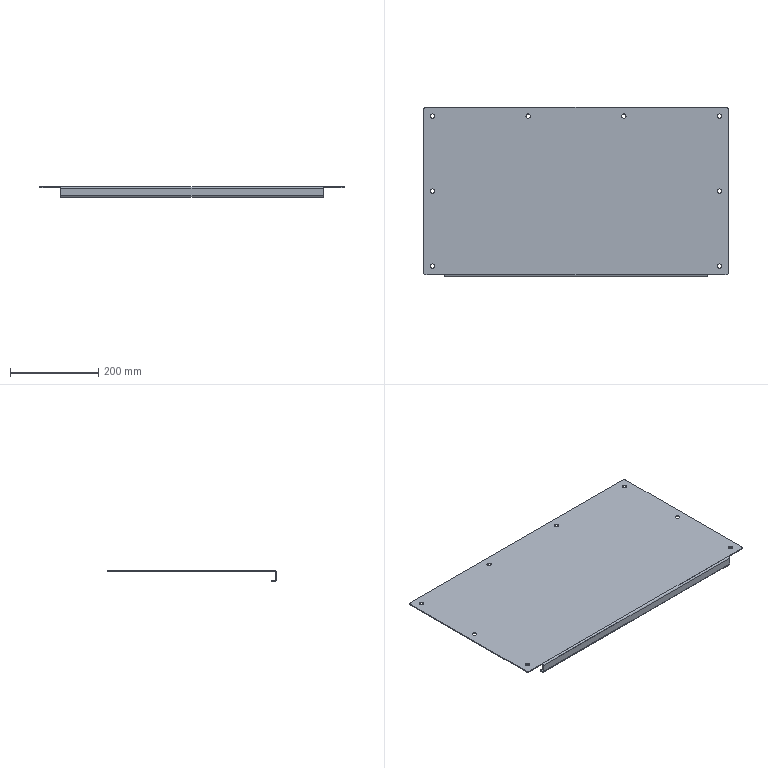Part | STEP file | 750038472 | 1 solid | 40 faces | box 690 x 384 x 24 mm | volume 562921 mm3 | cylinder 26 | plane 14 | commonest cylinder face diameters 10 x22 4 x2 8 x2
STEP:
#1=CARTESIAN_POINT('',(320.,360.,0.));
#2=VERTEX_POINT('',#1);
#3=CARTESIAN_POINT('',(330.,360.,0.));
#4=VERTEX_POINT('',#3);
#5=CARTESIAN_POINT('',(325.,360.,0.));
#6=DIRECTION('',(0.,0.,1.));
#7=DIRECTION('',(1.,0.,0.));
#8=AXIS2_PLACEMENT_3D('',#5,#6,#7);
#9=CIRCLE('',#8,5.);
#10=EDGE_CURVE('',#2,#4,#9,.T.);
#11=ORIENTED_EDGE('',*,*,#10,.F.);
#12=CARTESIAN_POINT('',(320.,360.,2.));
#13=VERTEX_POINT('',#12);
#14=CARTESIAN_POINT('',(320.,360.,-788.02));
#15=DIRECTION('',(0.,0.,1.));
#16=VECTOR('',#15,1000.);
#17=LINE('',#14,#16);
#18=EDGE_CURVE('',#2,#13,#17,.T.);
#19=ORIENTED_EDGE('',*,*,#18,.T.);
#20=CARTESIAN_POINT('',(330.,360.,2.));
#21=VERTEX_POINT('',#20);
#22=CARTESIAN_POINT('',(325.,360.,2.));
#23=DIRECTION('',(0.,0.,-1.));
#24=DIRECTION('',(1.,0.,0.));
#25=AXIS2_PLACEMENT_3D('',#22,#23,#24);
#26=CIRCLE('',#25,5.);
#27=EDGE_CURVE('',#21,#13,#26,.T.);
#28=ORIENTED_EDGE('',*,*,#27,.F.);
#29=CARTESIAN_POINT('',(330.,360.,-788.02));
#30=DIRECTION('',(0.,0.,1.));
#31=VECTOR('',#30,1000.);
#32=LINE('',#29,#31);
#33=EDGE_CURVE('',#4,#21,#32,.T.);
#34=ORIENTED_EDGE('',*,*,#33,.F.);
#35=EDGE_LOOP('',(#11,#19,#28,#34));
#36=FACE_OUTER_BOUND('',#35,.T.);
#37=CARTESIAN_POINT('',(325.,360.,-788.02));
#38=DIRECTION('',(0.,0.,1.));
#39=DIRECTION('',(1.,0.,0.));
#40=AXIS2_PLACEMENT_3D('',#37,#38,#39);
#41=CYLINDRICAL_SURFACE('',#40,5.);
#42=ADVANCED_FACE('',(#36),#41,.F.);
#43=CARTESIAN_POINT('',(320.,190.,0.));
#44=VERTEX_POINT('',#43);
#45=CARTESIAN_POINT('',(330.,190.,0.));
#46=VERTEX_POINT('',#45);
#47=CARTESIAN_POINT('',(325.,190.,0.));
#48=DIRECTION('',(0.,0.,1.));
#49=DIRECTION('',(1.,0.,0.));
#50=AXIS2_PLACEMENT_3D('',#47,#48,#49);
#51=CIRCLE('',#50,5.);
#52=EDGE_CURVE('',#44,#46,#51,.T.);
#53=ORIENTED_EDGE('',*,*,#52,.F.);
#54=CARTESIAN_POINT('',(320.,190.,2.));
#55=VERTEX_POINT('',#54);
#56=CARTESIAN_POINT('',(320.,190.,-788.02));
#57=DIRECTION('',(0.,0.,1.));
#58=VECTOR('',#57,1000.);
#59=LINE('',#56,#58);
#60=EDGE_CURVE('',#44,#55,#59,.T.);
#61=ORIENTED_EDGE('',*,*,#60,.T.);
#62=CARTESIAN_POINT('',(330.,190.,2.));
#63=VERTEX_POINT('',#62);
#64=CARTESIAN_POINT('',(325.,190.,2.));
#65=DIRECTION('',(0.,0.,-1.));
#66=DIRECTION('',(1.,0.,0.));
#67=AXIS2_PLACEMENT_3D('',#64,#65,#66);
#68=CIRCLE('',#67,5.);
#69=EDGE_CURVE('',#63,#55,#68,.T.);
#70=ORIENTED_EDGE('',*,*,#69,.F.);
#71=CARTESIAN_POINT('',(330.,190.,-788.02));
#72=DIRECTION('',(0.,0.,1.));
#73=VECTOR('',#72,1000.);
#74=LINE('',#71,#73);
#75=EDGE_CURVE('',#46,#63,#74,.T.);
#76=ORIENTED_EDGE('',*,*,#75,.F.);
#77=EDGE_LOOP('',(#53,#61,#70,#76));
#78=FACE_OUTER_BOUND('',#77,.T.);
#79=CARTESIAN_POINT('',(325.,190.,-788.02));
#80=DIRECTION('',(0.,0.,1.));
#81=DIRECTION('',(1.,0.,0.));
#82=AXIS2_PLACEMENT_3D('',#79,#80,#81);
#83=CYLINDRICAL_SURFACE('',#82,5.);
#84=ADVANCED_FACE('',(#78),#83,.F.);
#85=CARTESIAN_POINT('',(320.,20.,0.));
#86=VERTEX_POINT('',#85);
#87=CARTESIAN_POINT('',(330.,20.,0.));
#88=VERTEX_POINT('',#87);
#89=CARTESIAN_POINT('',(325.,20.,0.));
#90=DIRECTION('',(0.,0.,1.));
#91=DIRECTION('',(1.,0.,0.));
#92=AXIS2_PLACEMENT_3D('',#89,#90,#91);
#93=CIRCLE('',#92,5.);
#94=EDGE_CURVE('',#86,#88,#93,.T.);
#95=ORIENTED_EDGE('',*,*,#94,.F.);
#96=CARTESIAN_POINT('',(320.,20.,2.));
#97=VERTEX_POINT('',#96);
#98=CARTESIAN_POINT('',(320.,20.,-788.02));
#99=DIRECTION('',(0.,0.,1.));
#100=VECTOR('',#99,1000.);
#101=LINE('',#98,#100);
#102=EDGE_CURVE('',#86,#97,#101,.T.);
#103=ORIENTED_EDGE('',*,*,#102,.T.);
#104=CARTESIAN_POINT('',(330.,20.,2.));
#105=VERTEX_POINT('',#104);
#106=CARTESIAN_POINT('',(325.,20.,2.));
#107=DIRECTION('',(0.,0.,-1.));
#108=DIRECTION('',(1.,0.,0.));
#109=AXIS2_PLACEMENT_3D('',#106,#107,#108);
#110=CIRCLE('',#109,5.);
#111=EDGE_CURVE('',#105,#97,#110,.T.);
#112=ORIENTED_EDGE('',*,*,#111,.F.);
#113=CARTESIAN_POINT('',(330.,20.,-788.02));
#114=DIRECTION('',(0.,0.,1.));
#115=VECTOR('',#114,1000.);
#116=LINE('',#113,#115);
#117=EDGE_CURVE('',#88,#105,#116,.T.);
#118=ORIENTED_EDGE('',*,*,#117,.F.);
#119=EDGE_LOOP('',(#95,#103,#112,#118));
#120=FACE_OUTER_BOUND('',#119,.T.);
#121=CARTESIAN_POINT('',(325.,20.,-788.02));
#122=DIRECTION('',(0.,0.,1.));
#123=DIRECTION('',(1.,0.,0.));
#124=AXIS2_PLACEMENT_3D('',#121,#122,#123);
#125=CYLINDRICAL_SURFACE('',#124,5.);
#126=ADVANCED_FACE('',(#120),#125,.F.);
#127=CARTESIAN_POINT('',(103.333,360.,0.));
#128=VERTEX_POINT('',#127);
#129=CARTESIAN_POINT('',(113.333,360.,0.));
#130=VERTEX_POINT('',#129);
#131=CARTESIAN_POINT('',(108.333,360.,0.));
#132=DIRECTION('',(0.,0.,1.));
#133=DIRECTION('',(1.,0.,0.));
#134=AXIS2_PLACEMENT_3D('',#131,#132,#133);
#135=CIRCLE('',#134,5.);
#136=EDGE_CURVE('',#128,#130,#135,.T.);
#137=ORIENTED_EDGE('',*,*,#136,.F.);
#138=CARTESIAN_POINT('',(103.333,360.,2.));
#139=VERTEX_POINT('',#138);
#140=CARTESIAN_POINT('',(103.333,360.,-788.02));
#141=DIRECTION('',(0.,0.,1.));
#142=VECTOR('',#141,1000.);
#143=LINE('',#140,#142);
#144=EDGE_CURVE('',#128,#139,#143,.T.);
#145=ORIENTED_EDGE('',*,*,#144,.T.);
#146=CARTESIAN_POINT('',(113.333,360.,2.));
#147=VERTEX_POINT('',#146);
#148=CARTESIAN_POINT('',(108.333,360.,2.));
#149=DIRECTION('',(0.,0.,-1.));
#150=DIRECTION('',(1.,0.,0.));
#151=AXIS2_PLACEMENT_3D('',#148,#149,#150);
#152=CIRCLE('',#151,5.);
#153=EDGE_CURVE('',#147,#139,#152,.T.);
#154=ORIENTED_EDGE('',*,*,#153,.F.);
#155=CARTESIAN_POINT('',(113.333,360.,-788.02));
#156=DIRECTION('',(0.,0.,1.));
#157=VECTOR('',#156,1000.);
#158=LINE('',#155,#157);
#159=EDGE_CURVE('',#130,#147,#158,.T.);
#160=ORIENTED_EDGE('',*,*,#159,.F.);
#161=EDGE_LOOP('',(#137,#145,#154,#160));
#162=FACE_OUTER_BOUND('',#161,.T.);
#163=CARTESIAN_POINT('',(108.333,360.,-788.02));
#164=DIRECTION('',(0.,0.,1.));
#165=DIRECTION('',(1.,0.,0.));
#166=AXIS2_PLACEMENT_3D('',#163,#164,#165);
#167=CYLINDRICAL_SURFACE('',#166,5.);
#168=ADVANCED_FACE('',(#162),#167,.F.);
#169=CARTESIAN_POINT('',(-113.333,360.,0.));
#170=VERTEX_POINT('',#169);
#171=CARTESIAN_POINT('',(-103.333,360.,0.));
#172=VERTEX_POINT('',#171);
#173=CARTESIAN_POINT('',(-108.333,360.,0.));
#174=DIRECTION('',(0.,0.,1.));
#175=DIRECTION('',(1.,0.,0.));
#176=AXIS2_PLACEMENT_3D('',#173,#174,#175);
#177=CIRCLE('',#176,5.);
#178=EDGE_CURVE('',#170,#172,#177,.T.);
#179=ORIENTED_EDGE('',*,*,#178,.F.);
#180=CARTESIAN_POINT('',(-113.333,360.,2.));
#181=VERTEX_POINT('',#180);
#182=CARTESIAN_POINT('',(-113.333,360.,-788.02));
#183=DIRECTION('',(0.,0.,1.));
#184=VECTOR('',#183,1000.);
#185=LINE('',#182,#184);
#186=EDGE_CURVE('',#170,#181,#185,.T.);
#187=ORIENTED_EDGE('',*,*,#186,.T.);
#188=CARTESIAN_POINT('',(-103.333,360.,2.));
#189=VERTEX_POINT('',#188);
#190=CARTESIAN_POINT('',(-108.333,360.,2.));
#191=DIRECTION('',(0.,0.,-1.));
#192=DIRECTION('',(1.,0.,0.));
#193=AXIS2_PLACEMENT_3D('',#190,#191,#192);
#194=CIRCLE('',#193,5.);
#195=EDGE_CURVE('',#189,#181,#194,.T.);
#196=ORIENTED_EDGE('',*,*,#195,.F.);
#197=CARTESIAN_POINT('',(-103.333,360.,-788.02));
#198=DIRECTION('',(0.,0.,1.));
#199=VECTOR('',#198,1000.);
#200=LINE('',#197,#199);
#201=EDGE_CURVE('',#172,#189,#200,.T.);
#202=ORIENTED_EDGE('',*,*,#201,.F.);
#203=EDGE_LOOP('',(#179,#187,#196,#202));
#204=FACE_OUTER_BOUND('',#203,.T.);
#205=CARTESIAN_POINT('',(-108.333,360.,-788.02));
#206=DIRECTION('',(0.,0.,1.));
#207=DIRECTION('',(1.,0.,0.));
#208=AXIS2_PLACEMENT_3D('',#205,#206,#207);
#209=CYLINDRICAL_SURFACE('',#208,5.);
#210=ADVANCED_FACE('',(#204),#209,.F.);
#211=CARTESIAN_POINT('',(-330.,360.,0.));
#212=VERTEX_POINT('',#211);
#213=CARTESIAN_POINT('',(-320.,360.,0.));
#214=VERTEX_POINT('',#213);
#215=CARTESIAN_POINT('',(-325.,360.,0.));
#216=DIRECTION('',(0.,0.,1.));
#217=DIRECTION('',(1.,0.,0.));
#218=AXIS2_PLACEMENT_3D('',#215,#216,#217);
#219=CIRCLE('',#218,5.);
#220=EDGE_CURVE('',#212,#214,#219,.T.);
#221=ORIENTED_EDGE('',*,*,#220,.F.);
#222=CARTESIAN_POINT('',(-330.,360.,2.));
#223=VERTEX_POINT('',#222);
#224=CARTESIAN_POINT('',(-330.,360.,-788.02));
#225=DIRECTION('',(0.,0.,1.));
#226=VECTOR('',#225,1000.);
#227=LINE('',#224,#226);
#228=EDGE_CURVE('',#212,#223,#227,.T.);
#229=ORIENTED_EDGE('',*,*,#228,.T.);
#230=CARTESIAN_POINT('',(-320.,360.,2.));
#231=VERTEX_POINT('',#230);
#232=CARTESIAN_POINT('',(-325.,360.,2.));
#233=DIRECTION('',(0.,0.,-1.));
#234=DIRECTION('',(1.,0.,0.));
#235=AXIS2_PLACEMENT_3D('',#232,#233,#234);
#236=CIRCLE('',#235,5.);
#237=EDGE_CURVE('',#231,#223,#236,.T.);
#238=ORIENTED_EDGE('',*,*,#237,.F.);
#239=CARTESIAN_POINT('',(-320.,360.,-788.02));
#240=DIRECTION('',(0.,0.,1.));
#241=VECTOR('',#240,1000.);
#242=LINE('',#239,#241);
#243=EDGE_CURVE('',#214,#231,#242,.T.);
#244=ORIENTED_EDGE('',*,*,#243,.F.);
#245=EDGE_LOOP('',(#221,#229,#238,#244));
#246=FACE_OUTER_BOUND('',#245,.T.);
#247=CARTESIAN_POINT('',(-325.,360.,-788.02));
#248=DIRECTION('',(0.,0.,1.));
#249=DIRECTION('',(1.,0.,0.));
#250=AXIS2_PLACEMENT_3D('',#247,#248,#249);
#251=CYLINDRICAL_SURFACE('',#250,5.);
#252=ADVANCED_FACE('',(#246),#251,.F.);
#253=CARTESIAN_POINT('',(-330.,190.,0.));
#254=VERTEX_POINT('',#253);
#255=CARTESIAN_POINT('',(-320.,190.,0.));
#256=VERTEX_POINT('',#255);
#257=CARTESIAN_POINT('',(-325.,190.,0.));
#258=DIRECTION('',(0.,0.,1.));
#259=DIRECTION('',(1.,0.,0.));
#260=AXIS2_PLACEMENT_3D('',#257,#258,#259);
#261=CIRCLE('',#260,5.);
#262=EDGE_CURVE('',#254,#256,#261,.T.);
#263=ORIENTED_EDGE('',*,*,#262,.F.);
#264=CARTESIAN_POINT('',(-330.,190.,2.));
#265=VERTEX_POINT('',#264);
#266=CARTESIAN_POINT('',(-330.,190.,-788.02));
#267=DIRECTION('',(0.,0.,1.));
#268=VECTOR('',#267,1000.);
#269=LINE('',#266,#268);
#270=EDGE_CURVE('',#254,#265,#269,.T.);
#271=ORIENTED_EDGE('',*,*,#270,.T.);
#272=CARTESIAN_POINT('',(-320.,190.,2.));
#273=VERTEX_POINT('',#272);
#274=CARTESIAN_POINT('',(-325.,190.,2.));
#275=DIRECTION('',(0.,0.,-1.));
#276=DIRECTION('',(1.,0.,0.));
#277=AXIS2_PLACEMENT_3D('',#274,#275,#276);
#278=CIRCLE('',#277,5.);
#279=EDGE_CURVE('',#273,#265,#278,.T.);
#280=ORIENTED_EDGE('',*,*,#279,.F.);
#281=CARTESIAN_POINT('',(-320.,190.,-788.02));
#282=DIRECTION('',(0.,0.,1.));
#283=VECTOR('',#282,1000.);
#284=LINE('',#281,#283);
#285=EDGE_CURVE('',#256,#273,#284,.T.);
#286=ORIENTED_EDGE('',*,*,#285,.F.);
#287=EDGE_LOOP('',(#263,#271,#280,#286));
#288=FACE_OUTER_BOUND('',#287,.T.);
#289=CARTESIAN_POINT('',(-325.,190.,-788.02));
#290=DIRECTION('',(0.,0.,1.));
#291=DIRECTION('',(1.,0.,0.));
#292=AXIS2_PLACEMENT_3D('',#289,#290,#291);
#293=CYLINDRICAL_SURFACE('',#292,5.);
#294=ADVANCED_FACE('',(#288),#293,.F.);
#295=CARTESIAN_POINT('',(-330.,20.,0.));
#296=VERTEX_POINT('',#295);
#297=CARTESIAN_POINT('',(-320.,20.,0.));
#298=VERTEX_POINT('',#297);
#299=CARTESIAN_POINT('',(-325.,20.,0.));
#300=DIRECTION('',(0.,0.,1.));
#301=DIRECTION('',(1.,0.,0.));
#302=AXIS2_PLACEMENT_3D('',#299,#300,#301);
#303=CIRCLE('',#302,5.);
#304=EDGE_CURVE('',#296,#298,#303,.T.);
#305=ORIENTED_EDGE('',*,*,#304,.F.);
#306=CARTESIAN_POINT('',(-330.,20.,2.));
#307=VERTEX_POINT('',#306);
#308=CARTESIAN_POINT('',(-330.,20.,-788.02));
#309=DIRECTION('',(0.,0.,1.));
#310=VECTOR('',#309,1000.);
#311=LINE('',#308,#310);
#312=EDGE_CURVE('',#296,#307,#311,.T.);
#313=ORIENTED_EDGE('',*,*,#312,.T.);
#314=CARTESIAN_POINT('',(-320.,20.,2.));
#315=VERTEX_POINT('',#314);
#316=CARTESIAN_POINT('',(-325.,20.,2.));
#317=DIRECTION('',(0.,0.,-1.));
#318=DIRECTION('',(1.,0.,0.));
#319=AXIS2_PLACEMENT_3D('',#316,#317,#318);
#320=CIRCLE('',#319,5.);
#321=EDGE_CURVE('',#315,#307,#320,.T.);
#322=ORIENTED_EDGE('',*,*,#321,.F.);
#323=CARTESIAN_POINT('',(-320.,20.,-788.02));
#324=DIRECTION('',(0.,0.,1.));
#325=VECTOR('',#324,1000.);
#326=LINE('',#323,#325);
#327=EDGE_CURVE('',#298,#315,#326,.T.);
#328=ORIENTED_EDGE('',*,*,#327,.F.);
#329=EDGE_LOOP('',(#305,#313,#322,#328));
#330=FACE_OUTER_BOUND('',#329,.T.);
#331=CARTESIAN_POINT('',(-325.,20.,-788.02));
#332=DIRECTION('',(0.,0.,1.));
#333=DIRECTION('',(1.,0.,0.));
#334=AXIS2_PLACEMENT_3D('',#331,#332,#333);
#335=CYLINDRICAL_SURFACE('',#334,5.);
#336=ADVANCED_FACE('',(#330),#335,.F.);
#337=CARTESIAN_POINT('',(345.,5.,2.));
#338=VERTEX_POINT('',#337);
#339=CARTESIAN_POINT('',(345.,375.,2.));
#340=VERTEX_POINT('',#339);
#341=CARTESIAN_POINT('',(345.,0.,2.));
#342=DIRECTION('',(0.,1.,0.));
#343=VECTOR('',#342,1000.);
#344=LINE('',#341,#343);
#345=EDGE_CURVE('',#338,#340,#344,.T.);
#346=ORIENTED_EDGE('',*,*,#345,.T.);
#347=CARTESIAN_POINT('',(340.,380.,2.));
#348=VERTEX_POINT('',#347);
#349=CARTESIAN_POINT('',(340.,375.,2.));
#350=DIRECTION('',(0.,0.,1.));
#351=DIRECTION('',(-1.,0.,0.));
#352=AXIS2_PLACEMENT_3D('',#349,#350,#351);
#353=CIRCLE('',#352,5.);
#354=EDGE_CURVE('',#340,#348,#353,.T.);
#355=ORIENTED_EDGE('',*,*,#354,.T.);
#356=CARTESIAN_POINT('',(-340.,380.,2.));
#357=VERTEX_POINT('',#356);
#358=CARTESIAN_POINT('',(0.,380.,2.));
#359=DIRECTION('',(-1.,0.,0.));
#360=VECTOR('',#359,1000.);
#361=LINE('',#358,#360);
#362=EDGE_CURVE('',#348,#357,#361,.T.);
#363=ORIENTED_EDGE('',*,*,#362,.T.);
#364=CARTESIAN_POINT('',(-345.,375.,2.));
#365=VERTEX_POINT('',#364);
#366=CARTESIAN_POINT('',(-340.,375.,2.));
#367=DIRECTION('',(0.,0.,1.));
#368=DIRECTION('',(-1.,0.,0.));
#369=AXIS2_PLACEMENT_3D('',#366,#367,#368);
#370=CIRCLE('',#369,5.);
#371=EDGE_CURVE('',#357,#365,#370,.T.);
#372=ORIENTED_EDGE('',*,*,#371,.T.);
#373=CARTESIAN_POINT('',(-345.,5.,2.));
#374=VERTEX_POINT('',#373);
#375=CARTESIAN_POINT('',(-345.,0.,2.));
#376=DIRECTION('',(0.,-1.,0.));
#377=VECTOR('',#376,1000.);
#378=LINE('',#375,#377);
#379=EDGE_CURVE('',#365,#374,#378,.T.);
#380=ORIENTED_EDGE('',*,*,#379,.T.);
#381=CARTESIAN_POINT('',(-340.,0.,2.));
#382=VERTEX_POINT('',#381);
#383=CARTESIAN_POINT('',(-340.,5.,2.));
#384=DIRECTION('',(0.,0.,1.));
#385=DIRECTION('',(-1.,0.,0.));
#386=AXIS2_PLACEMENT_3D('',#383,#384,#385);
#387=CIRCLE('',#386,5.);
#388=EDGE_CURVE('',#374,#382,#387,.T.);
#389=ORIENTED_EDGE('',*,*,#388,.T.);
#390=CARTESIAN_POINT('',(-298.,0.,2.));
#391=VERTEX_POINT('',#390);
#392=CARTESIAN_POINT('',(0.,0.,2.));
#393=DIRECTION('',(1.,0.,0.));
#394=VECTOR('',#393,1000.);
#395=LINE('',#392,#394);
#396=EDGE_CURVE('',#382,#391,#395,.T.);
#397=ORIENTED_EDGE('',*,*,#396,.T.);
#398=CARTESIAN_POINT('',(298.,0.,2.));
#399=VERTEX_POINT('',#398);
#400=CARTESIAN_POINT('',(0.,0.,2.));
#401=DIRECTION('',(1.,0.,0.));
#402=VECTOR('',#401,1000.);
#403=LINE('',#400,#402);
#404=EDGE_CURVE('',#391,#399,#403,.T.);
#405=ORIENTED_EDGE('',*,*,#404,.T.);
#406=CARTESIAN_POINT('',(340.,0.,2.));
#407=VERTEX_POINT('',#406);
#408=CARTESIAN_POINT('',(0.,0.,2.));
#409=DIRECTION('',(1.,0.,0.));
#410=VECTOR('',#409,1000.);
#411=LINE('',#408,#410);
#412=EDGE_CURVE('',#399,#407,#411,.T.);
#413=ORIENTED_EDGE('',*,*,#412,.T.);
#414=CARTESIAN_POINT('',(340.,5.,2.));
#415=DIRECTION('',(0.,0.,1.));
#416=DIRECTION('',(-1.,0.,0.));
#417=AXIS2_PLACEMENT_3D('',#414,#415,#416);
#418=CIRCLE('',#417,5.);
#419=EDGE_CURVE('',#407,#338,#418,.T.);
#420=ORIENTED_EDGE('',*,*,#419,.T.);
#421=EDGE_LOOP('',(#346,#355,#363,#372,#380,#389,#397,#405,#413,#420));
#422=FACE_OUTER_BOUND('',#421,.T.);
#423=ORIENTED_EDGE('',*,*,#27,.T.);
#424=CARTESIAN_POINT('',(325.,360.,2.));
#425=DIRECTION('',(0.,0.,-1.));
#426=DIRECTION('',(1.,0.,0.));
#427=AXIS2_PLACEMENT_3D('',#424,#425,#426);
#428=CIRCLE('',#427,5.);
#429=EDGE_CURVE('',#13,#21,#428,.T.);
#430=ORIENTED_EDGE('',*,*,#429,.T.);
#431=EDGE_LOOP('',(#423,#430));
#432=FACE_BOUND('',#431,.T.);
#433=ORIENTED_EDGE('',*,*,#69,.T.);
#434=CARTESIAN_POINT('',(325.,190.,2.));
#435=DIRECTION('',(0.,0.,-1.));
#436=DIRECTION('',(1.,0.,0.));
#437=AXIS2_PLACEMENT_3D('',#434,#435,#436);
#438=CIRCLE('',#437,5.);
#439=EDGE_CURVE('',#55,#63,#438,.T.);
#440=ORIENTED_EDGE('',*,*,#439,.T.);
#441=EDGE_LOOP('',(#433,#440));
#442=FACE_BOUND('',#441,.T.);
#443=ORIENTED_EDGE('',*,*,#111,.T.);
#444=CARTESIAN_POINT('',(325.,20.,2.));
#445=DIRECTION('',(0.,0.,-1.));
#446=DIRECTION('',(1.,0.,0.));
#447=AXIS2_PLACEMENT_3D('',#444,#445,#446);
#448=CIRCLE('',#447,5.);
#449=EDGE_CURVE('',#97,#105,#448,.T.);
#450=ORIENTED_EDGE('',*,*,#449,.T.);
#451=EDGE_LOOP('',(#443,#450));
#452=FACE_BOUND('',#451,.T.);
#453=ORIENTED_EDGE('',*,*,#153,.T.);
#454=CARTESIAN_POINT('',(108.333,360.,2.));
#455=DIRECTION('',(0.,0.,-1.));
#456=DIRECTION('',(1.,0.,0.));
#457=AXIS2_PLACEMENT_3D('',#454,#455,#456);
#458=CIRCLE('',#457,5.);
#459=EDGE_CURVE('',#139,#147,#458,.T.);
#460=ORIENTED_EDGE('',*,*,#459,.T.);
#461=EDGE_LOOP('',(#453,#460));
#462=FACE_BOUND('',#461,.T.);
#463=ORIENTED_EDGE('',*,*,#195,.T.);
#464=CARTESIAN_POINT('',(-108.333,360.,2.));
#465=DIRECTION('',(0.,0.,-1.));
#466=DIRECTION('',(1.,0.,0.));
#467=AXIS2_PLACEMENT_3D('',#464,#465,#466);
#468=CIRCLE('',#467,5.);
#469=EDGE_CURVE('',#181,#189,#468,.T.);
#470=ORIENTED_EDGE('',*,*,#469,.T.);
#471=EDGE_LOOP('',(#463,#470));
#472=FACE_BOUND('',#471,.T.);
#473=ORIENTED_EDGE('',*,*,#237,.T.);
#474=CARTESIAN_POINT('',(-325.,360.,2.));
#475=DIRECTION('',(0.,0.,-1.));
#476=DIRECTION('',(1.,0.,0.));
#477=AXIS2_PLACEMENT_3D('',#474,#475,#476);
#478=CIRCLE('',#477,5.);
#479=EDGE_CURVE('',#223,#231,#478,.T.);
#480=ORIENTED_EDGE('',*,*,#479,.T.);
#481=EDGE_LOOP('',(#473,#480));
#482=FACE_BOUND('',#481,.T.);
#483=ORIENTED_EDGE('',*,*,#279,.T.);
#484=CARTESIAN_POINT('',(-325.,190.,2.));
#485=DIRECTION('',(0.,0.,-1.));
#486=DIRECTION('',(1.,0.,0.));
#487=AXIS2_PLACEMENT_3D('',#484,#485,#486);
#488=CIRCLE('',#487,5.);
#489=EDGE_CURVE('',#265,#273,#488,.T.);
#490=ORIENTED_EDGE('',*,*,#489,.T.);
#491=EDGE_LOOP('',(#483,#490));
#492=FACE_BOUND('',#491,.T.);
#493=ORIENTED_EDGE('',*,*,#321,.T.);
#494=CARTESIAN_POINT('',(-325.,20.,2.));
#495=DIRECTION('',(0.,0.,-1.));
#496=DIRECTION('',(1.,0.,0.));
#497=AXIS2_PLACEMENT_3D('',#494,#495,#496);
#498=CIRCLE('',#497,5.);
#499=EDGE_CURVE('',#307,#315,#498,.T.);
#500=ORIENTED_EDGE('',*,*,#499,.T.);
#501=EDGE_LOOP('',(#493,#500));
#502=FACE_BOUND('',#501,.T.);
#503=CARTESIAN_POINT('',(0.,0.,2.));
#504=DIRECTION('',(0.,0.,1.));
#505=DIRECTION('',(1.,0.,0.));
#506=AXIS2_PLACEMENT_3D('',#503,#504,#505);
#507=PLANE('',#506);
#508=ADVANCED_FACE('',(#422,#432,#442,#452,#462,#472,#482,#492,#502),#507,.T.);
#509=CARTESIAN_POINT('',(345.,375.,0.));
#510=VERTEX_POINT('',#509);
#511=CARTESIAN_POINT('',(340.,380.,0.));
#512=VERTEX_POINT('',#511);
#513=CARTESIAN_POINT('',(340.,375.,0.));
#514=DIRECTION('',(0.,0.,1.));
#515=DIRECTION('',(-1.,0.,0.));
#516=AXIS2_PLACEMENT_3D('',#513,#514,#515);
#517=CIRCLE('',#516,5.);
#518=EDGE_CURVE('',#510,#512,#517,.T.);
#519=ORIENTED_EDGE('',*,*,#518,.T.);
#520=CARTESIAN_POINT('',(340.,380.,2.));
#521=DIRECTION('',(0.,0.,1.));
#522=VECTOR('',#521,1000.);
#523=LINE('',#520,#522);
#524=EDGE_CURVE('',#512,#348,#523,.T.);
#525=ORIENTED_EDGE('',*,*,#524,.T.);
#526=ORIENTED_EDGE('',*,*,#354,.F.);
#527=CARTESIAN_POINT('',(345.,375.,2.));
#528=DIRECTION('',(0.,0.,-1.));
#529=VECTOR('',#528,1000.);
#530=LINE('',#527,#529);
#531=EDGE_CURVE('',#340,#510,#530,.T.);
#532=ORIENTED_EDGE('',*,*,#531,.T.);
#533=EDGE_LOOP('',(#519,#525,#526,#532));
#534=FACE_OUTER_BOUND('',#533,.T.);
#535=CARTESIAN_POINT('',(340.,375.,2.));
#536=DIRECTION('',(0.,0.,-1.));
#537=DIRECTION('',(-1.,0.,0.));
#538=AXIS2_PLACEMENT_3D('',#535,#536,#537);
#539=CYLINDRICAL_SURFACE('',#538,5.);
#540=ADVANCED_FACE('',(#534),#539,.T.);
#541=CARTESIAN_POINT('',(345.,5.,0.));
#542=VERTEX_POINT('',#541);
#543=CARTESIAN_POINT('',(345.,5.,2.));
#544=DIRECTION('',(0.,0.,1.));
#545=VECTOR('',#544,1000.);
#546=LINE('',#543,#545);
#547=EDGE_CURVE('',#542,#338,#546,.T.);
#548=ORIENTED_EDGE('',*,*,#547,.F.);
#549=CARTESIAN_POINT('',(345.,0.,0.));
#550=DIRECTION('',(0.,-1.,0.));
#551=VECTOR('',#550,1000.);
#552=LINE('',#549,#551);
#553=EDGE_CURVE('',#510,#542,#552,.T.);
#554=ORIENTED_EDGE('',*,*,#553,.F.);
#555=ORIENTED_EDGE('',*,*,#531,.F.);
#556=ORIENTED_EDGE('',*,*,#345,.F.);
#557=EDGE_LOOP('',(#548,#554,#555,#556));
#558=FACE_OUTER_BOUND('',#557,.T.);
#559=CARTESIAN_POINT('',(345.,0.,2.));
#560=DIRECTION('',(-1.,0.,0.));
#561=DIRECTION('',(0.,-1.,0.));
#562=AXIS2_PLACEMENT_3D('',#559,#560,#561);
#563=PLANE('',#562);
#564=ADVANCED_FACE('',(#558),#563,.F.);
#565=CARTESIAN_POINT('',(340.,0.,0.));
#566=VERTEX_POINT('',#565);
#567=CARTESIAN_POINT('',(340.,5.,0.));
#568=DIRECTION('',(0.,0.,1.));
#569=DIRECTION('',(-1.,0.,0.));
#570=AXIS2_PLACEMENT_3D('',#567,#568,#569);
#571=CIRCLE('',#570,5.);
#572=EDGE_CURVE('',#566,#542,#571,.T.);
#573=ORIENTED_EDGE('',*,*,#572,.T.);
#574=ORIENTED_EDGE('',*,*,#547,.T.);
#575=ORIENTED_EDGE('',*,*,#419,.F.);
#576=CARTESIAN_POINT('',(340.,0.,2.));
#577=DIRECTION('',(0.,0.,-1.));
#578=VECTOR('',#577,1000.);
#579=LINE('',#576,#578);
#580=EDGE_CURVE('',#407,#566,#579,.T.);
#581=ORIENTED_EDGE('',*,*,#580,.T.);
#582=EDGE_LOOP('',(#573,#574,#575,#581));
#583=FACE_OUTER_BOUND('',#582,.T.);
#584=CARTESIAN_POINT('',(340.,5.,2.));
#585=DIRECTION('',(0.,0.,-1.));
#586=DIRECTION('',(-1.,0.,0.));
#587=AXIS2_PLACEMENT_3D('',#584,#585,#586);
#588=CYLINDRICAL_SURFACE('',#587,5.);
#589=ADVANCED_FACE('',(#583),#588,.T.);
#590=ORIENTED_EDGE('',*,*,#580,.F.);
#591=ORIENTED_EDGE('',*,*,#412,.F.);
#592=CARTESIAN_POINT('',(298.,0.,0.));
#593=VERTEX_POINT('',#592);
#594=CARTESIAN_POINT('',(298.,0.,2.));
#595=DIRECTION('',(0.,0.,1.));
#596=VECTOR('',#595,1000.);
#597=LINE('',#594,#596);
#598=EDGE_CURVE('',#593,#399,#597,.T.);
#599=ORIENTED_EDGE('',*,*,#598,.F.);
#600=CARTESIAN_POINT('',(-345.,0.,0.));
#601=DIRECTION('',(-1.,0.,0.));
#602=VECTOR('',#601,1000.);
#603=LINE('',#600,#602);
#604=EDGE_CURVE('',#566,#593,#603,.T.);
#605=ORIENTED_EDGE('',*,*,#604,.F.);
#606=EDGE_LOOP('',(#590,#591,#599,#605));
#607=FACE_OUTER_BOUND('',#606,.T.);
#608=CARTESIAN_POINT('',(-345.,0.,2.));
#609=DIRECTION('',(0.,1.,0.));
#610=DIRECTION('',(0.,0.,1.));
#611=AXIS2_PLACEMENT_3D('',#608,#609,#610);
#612=PLANE('',#611);
#613=ADVANCED_FACE('',(#607),#612,.F.);
#614=CARTESIAN_POINT('',(298.,-4.,-2.));
#615=VERTEX_POINT('',#614);
#616=CARTESIAN_POINT('',(298.,0.,-2.));
#617=DIRECTION('',(-1.,0.,0.));
#618=DIRECTION('',(0.,0.,1.));
#619=AXIS2_PLACEMENT_3D('',#616,#617,#618);
#620=CIRCLE('',#619,4.);
#621=EDGE_CURVE('',#615,#399,#620,.T.);
#622=ORIENTED_EDGE('',*,*,#621,.T.);
#623=ORIENTED_EDGE('',*,*,#404,.F.);
#624=CARTESIAN_POINT('',(-298.,-4.,-2.));
#625=VERTEX_POINT('',#624);
#626=CARTESIAN_POINT('',(-298.,0.,-2.));
#627=DIRECTION('',(1.,0.,0.));
#628=DIRECTION('',(0.,0.,1.));
#629=AXIS2_PLACEMENT_3D('',#626,#627,#628);
#630=CIRCLE('',#629,4.);
#631=EDGE_CURVE('',#391,#625,#630,.T.);
#632=ORIENTED_EDGE('',*,*,#631,.T.);
#633=CARTESIAN_POINT('',(298.,-4.,-2.));
#634=DIRECTION('',(1.,0.,0.));
#635=VECTOR('',#634,1000.);
#636=LINE('',#633,#635);
#637=EDGE_CURVE('',#625,#615,#636,.T.);
#638=ORIENTED_EDGE('',*,*,#637,.T.);
#639=EDGE_LOOP('',(#622,#623,#632,#638));
#640=FACE_OUTER_BOUND('',#639,.T.);
#641=CARTESIAN_POINT('',(298.,0.,-2.));
#642=DIRECTION('',(-1.,0.,0.));
#643=DIRECTION('',(0.,0.,1.));
#644=AXIS2_PLACEMENT_3D('',#641,#642,#643);
#645=CYLINDRICAL_SURFACE('',#644,4.);
#646=ADVANCED_FACE('',(#640),#645,.T.);
#647=CARTESIAN_POINT('',(-340.,0.,0.));
#648=VERTEX_POINT('',#647);
#649=CARTESIAN_POINT('',(-340.,0.,2.));
#650=DIRECTION('',(0.,0.,1.));
#651=VECTOR('',#650,1000.);
#652=LINE('',#649,#651);
#653=EDGE_CURVE('',#648,#382,#652,.T.);
#654=ORIENTED_EDGE('',*,*,#653,.F.);
#655=CARTESIAN_POINT('',(-298.,0.,0.));
#656=VERTEX_POINT('',#655);
#657=CARTESIAN_POINT('',(-345.,0.,0.));
#658=DIRECTION('',(-1.,0.,0.));
#659=VECTOR('',#658,1000.);
#660=LINE('',#657,#659);
#661=EDGE_CURVE('',#656,#648,#660,.T.);
#662=ORIENTED_EDGE('',*,*,#661,.F.);
#663=CARTESIAN_POINT('',(-298.,0.,2.));
#664=DIRECTION('',(0.,0.,-1.));
#665=VECTOR('',#664,1000.);
#666=LINE('',#663,#665);
#667=EDGE_CURVE('',#391,#656,#666,.T.);
#668=ORIENTED_EDGE('',*,*,#667,.F.);
#669=ORIENTED_EDGE('',*,*,#396,.F.);
#670=EDGE_LOOP('',(#654,#662,#668,#669));
#671=FACE_OUTER_BOUND('',#670,.T.);
#672=CARTESIAN_POINT('',(-345.,0.,2.));
#673=DIRECTION('',(0.,1.,0.));
#674=DIRECTION('',(0.,0.,1.));
#675=AXIS2_PLACEMENT_3D('',#672,#673,#674);
#676=PLANE('',#675);
#677=ADVANCED_FACE('',(#671),#676,.F.);
#678=CARTESIAN_POINT('',(-345.,5.,0.));
#679=VERTEX_POINT('',#678);
#680=CARTESIAN_POINT('',(-340.,5.,0.));
#681=DIRECTION('',(0.,0.,1.));
#682=DIRECTION('',(-1.,0.,0.));
#683=AXIS2_PLACEMENT_3D('',#680,#681,#682);
#684=CIRCLE('',#683,5.);
#685=EDGE_CURVE('',#679,#648,#684,.T.);
#686=ORIENTED_EDGE('',*,*,#685,.T.);
#687=ORIENTED_EDGE('',*,*,#653,.T.);
#688=ORIENTED_EDGE('',*,*,#388,.F.);
#689=CARTESIAN_POINT('',(-345.,5.,2.));
#690=DIRECTION('',(0.,0.,-1.));
#691=VECTOR('',#690,1000.);
#692=LINE('',#689,#691);
#693=EDGE_CURVE('',#374,#679,#692,.T.);
#694=ORIENTED_EDGE('',*,*,#693,.T.);
#695=EDGE_LOOP('',(#686,#687,#688,#694));
#696=FACE_OUTER_BOUND('',#695,.T.);
#697=CARTESIAN_POINT('',(-340.,5.,2.));
#698=DIRECTION('',(0.,0.,-1.));
#699=DIRECTION('',(-1.,0.,0.));
#700=AXIS2_PLACEMENT_3D('',#697,#698,#699);
#701=CYLINDRICAL_SURFACE('',#700,5.);
#702=ADVANCED_FACE('',(#696),#701,.T.);
#703=CARTESIAN_POINT('',(-345.,375.,0.));
#704=VERTEX_POINT('',#703);
#705=CARTESIAN_POINT('',(-345.,375.,2.));
#706=DIRECTION('',(0.,0.,1.));
#707=VECTOR('',#706,1000.);
#708=LINE('',#705,#707);
#709=EDGE_CURVE('',#704,#365,#708,.T.);
#710=ORIENTED_EDGE('',*,*,#709,.F.);
#711=CARTESIAN_POINT('',(-345.,380.,0.));
#712=DIRECTION('',(0.,1.,0.));
#713=VECTOR('',#712,1000.);
#714=LINE('',#711,#713);
#715=EDGE_CURVE('',#679,#704,#714,.T.);
#716=ORIENTED_EDGE('',*,*,#715,.F.);
#717=ORIENTED_EDGE('',*,*,#693,.F.);
#718=ORIENTED_EDGE('',*,*,#379,.F.);
#719=EDGE_LOOP('',(#710,#716,#717,#718));
#720=FACE_OUTER_BOUND('',#719,.T.);
#721=CARTESIAN_POINT('',(-345.,380.,2.));
#722=DIRECTION('',(1.,0.,0.));
#723=DIRECTION('',(0.,1.,0.));
#724=AXIS2_PLACEMENT_3D('',#721,#722,#723);
#725=PLANE('',#724);
#726=ADVANCED_FACE('',(#720),#725,.F.);
#727=CARTESIAN_POINT('',(-340.,380.,0.));
#728=VERTEX_POINT('',#727);
#729=CARTESIAN_POINT('',(-340.,375.,0.));
#730=DIRECTION('',(0.,0.,1.));
#731=DIRECTION('',(-1.,0.,0.));
#732=AXIS2_PLACEMENT_3D('',#729,#730,#731);
#733=CIRCLE('',#732,5.);
#734=EDGE_CURVE('',#728,#704,#733,.T.);
#735=ORIENTED_EDGE('',*,*,#734,.T.);
#736=ORIENTED_EDGE('',*,*,#709,.T.);
#737=ORIENTED_EDGE('',*,*,#371,.F.);
#738=CARTESIAN_POINT('',(-340.,380.,2.));
#739=DIRECTION('',(0.,0.,-1.));
#740=VECTOR('',#739,1000.);
#741=LINE('',#738,#740);
#742=EDGE_CURVE('',#357,#728,#741,.T.);
#743=ORIENTED_EDGE('',*,*,#742,.T.);
#744=EDGE_LOOP('',(#735,#736,#737,#743));
#745=FACE_OUTER_BOUND('',#744,.T.);
#746=CARTESIAN_POINT('',(-340.,375.,2.));
#747=DIRECTION('',(0.,0.,-1.));
#748=DIRECTION('',(-1.,0.,0.));
#749=AXIS2_PLACEMENT_3D('',#746,#747,#748);
#750=CYLINDRICAL_SURFACE('',#749,5.);
#751=ADVANCED_FACE('',(#745),#750,.T.);
#752=ORIENTED_EDGE('',*,*,#742,.F.);
#753=ORIENTED_EDGE('',*,*,#362,.F.);
#754=ORIENTED_EDGE('',*,*,#524,.F.);
#755=CARTESIAN_POINT('',(345.,380.,0.));
#756=DIRECTION('',(1.,0.,0.));
#757=VECTOR('',#756,1000.);
#758=LINE('',#755,#757);
#759=EDGE_CURVE('',#728,#512,#758,.T.);
#760=ORIENTED_EDGE('',*,*,#759,.F.);
#761=EDGE_LOOP('',(#752,#753,#754,#760));
#762=FACE_OUTER_BOUND('',#761,.T.);
#763=CARTESIAN_POINT('',(345.,380.,2.));
#764=DIRECTION('',(0.,-1.,0.));
#765=DIRECTION('',(0.,0.,-1.));
#766=AXIS2_PLACEMENT_3D('',#763,#764,#765);
#767=PLANE('',#766);
#768=ADVANCED_FACE('',(#762),#767,.F.);
#769=ORIENTED_EDGE('',*,*,#18,.F.);
#770=CARTESIAN_POINT('',(325.,360.,0.));
#771=DIRECTION('',(0.,0.,1.));
#772=DIRECTION('',(1.,0.,0.));
#773=AXIS2_PLACEMENT_3D('',#770,#771,#772);
#774=CIRCLE('',#773,5.);
#775=EDGE_CURVE('',#4,#2,#774,.T.);
#776=ORIENTED_EDGE('',*,*,#775,.F.);
#777=ORIENTED_EDGE('',*,*,#33,.T.);
#778=ORIENTED_EDGE('',*,*,#429,.F.);
#779=EDGE_LOOP('',(#769,#776,#777,#778));
#780=FACE_OUTER_BOUND('',#779,.T.);
#781=CARTESIAN_POINT('',(325.,360.,-788.02));
#782=DIRECTION('',(0.,0.,1.));
#783=DIRECTION('',(1.,0.,0.));
#784=AXIS2_PLACEMENT_3D('',#781,#782,#783);
#785=CYLINDRICAL_SURFACE('',#784,5.);
#786=ADVANCED_FACE('',(#780),#785,.F.);
#787=ORIENTED_EDGE('',*,*,#60,.F.);
#788=CARTESIAN_POINT('',(325.,190.,0.));
#789=DIRECTION('',(0.,0.,1.));
#790=DIRECTION('',(1.,0.,0.));
#791=AXIS2_PLACEMENT_3D('',#788,#789,#790);
#792=CIRCLE('',#791,5.);
#793=EDGE_CURVE('',#46,#44,#792,.T.);
#794=ORIENTED_EDGE('',*,*,#793,.F.);
#795=ORIENTED_EDGE('',*,*,#75,.T.);
#796=ORIENTED_EDGE('',*,*,#439,.F.);
#797=EDGE_LOOP('',(#787,#794,#795,#796));
#798=FACE_OUTER_BOUND('',#797,.T.);
#799=CARTESIAN_POINT('',(325.,190.,-788.02));
#800=DIRECTION('',(0.,0.,1.));
#801=DIRECTION('',(1.,0.,0.));
#802=AXIS2_PLACEMENT_3D('',#799,#800,#801);
#803=CYLINDRICAL_SURFACE('',#802,5.);
#804=ADVANCED_FACE('',(#798),#803,.F.);
#805=ORIENTED_EDGE('',*,*,#102,.F.);
#806=CARTESIAN_POINT('',(325.,20.,0.));
#807=DIRECTION('',(0.,0.,1.));
#808=DIRECTION('',(1.,0.,0.));
#809=AXIS2_PLACEMENT_3D('',#806,#807,#808);
#810=CIRCLE('',#809,5.);
#811=EDGE_CURVE('',#88,#86,#810,.T.);
#812=ORIENTED_EDGE('',*,*,#811,.F.);
#813=ORIENTED_EDGE('',*,*,#117,.T.);
#814=ORIENTED_EDGE('',*,*,#449,.F.);
#815=EDGE_LOOP('',(#805,#812,#813,#814));
#816=FACE_OUTER_BOUND('',#815,.T.);
#817=CARTESIAN_POINT('',(325.,20.,-788.02));
#818=DIRECTION('',(0.,0.,1.));
#819=DIRECTION('',(1.,0.,0.));
#820=AXIS2_PLACEMENT_3D('',#817,#818,#819);
#821=CYLINDRICAL_SURFACE('',#820,5.);
#822=ADVANCED_FACE('',(#816),#821,.F.);
#823=ORIENTED_EDGE('',*,*,#144,.F.);
#824=CARTESIAN_POINT('',(108.333,360.,0.));
#825=DIRECTION('',(0.,0.,1.));
#826=DIRECTION('',(1.,0.,0.));
#827=AXIS2_PLACEMENT_3D('',#824,#825,#826);
#828=CIRCLE('',#827,5.);
#829=EDGE_CURVE('',#130,#128,#828,.T.);
#830=ORIENTED_EDGE('',*,*,#829,.F.);
#831=ORIENTED_EDGE('',*,*,#159,.T.);
#832=ORIENTED_EDGE('',*,*,#459,.F.);
#833=EDGE_LOOP('',(#823,#830,#831,#832));
#834=FACE_OUTER_BOUND('',#833,.T.);
#835=CARTESIAN_POINT('',(108.333,360.,-788.02));
#836=DIRECTION('',(0.,0.,1.));
#837=DIRECTION('',(1.,0.,0.));
#838=AXIS2_PLACEMENT_3D('',#835,#836,#837);
#839=CYLINDRICAL_SURFACE('',#838,5.);
#840=ADVANCED_FACE('',(#834),#839,.F.);
#841=ORIENTED_EDGE('',*,*,#186,.F.);
#842=CARTESIAN_POINT('',(-108.333,360.,0.));
#843=DIRECTION('',(0.,0.,1.));
#844=DIRECTION('',(1.,0.,0.));
#845=AXIS2_PLACEMENT_3D('',#842,#843,#844);
#846=CIRCLE('',#845,5.);
#847=EDGE_CURVE('',#172,#170,#846,.T.);
#848=ORIENTED_EDGE('',*,*,#847,.F.);
#849=ORIENTED_EDGE('',*,*,#201,.T.);
#850=ORIENTED_EDGE('',*,*,#469,.F.);
#851=EDGE_LOOP('',(#841,#848,#849,#850));
#852=FACE_OUTER_BOUND('',#851,.T.);
#853=CARTESIAN_POINT('',(-108.333,360.,-788.02));
#854=DIRECTION('',(0.,0.,1.));
#855=DIRECTION('',(1.,0.,0.));
#856=AXIS2_PLACEMENT_3D('',#853,#854,#855);
#857=CYLINDRICAL_SURFACE('',#856,5.);
#858=ADVANCED_FACE('',(#852),#857,.F.);
#859=ORIENTED_EDGE('',*,*,#228,.F.);
#860=CARTESIAN_POINT('',(-325.,360.,0.));
#861=DIRECTION('',(0.,0.,1.));
#862=DIRECTION('',(1.,0.,0.));
#863=AXIS2_PLACEMENT_3D('',#860,#861,#862);
#864=CIRCLE('',#863,5.);
#865=EDGE_CURVE('',#214,#212,#864,.T.);
#866=ORIENTED_EDGE('',*,*,#865,.F.);
#867=ORIENTED_EDGE('',*,*,#243,.T.);
#868=ORIENTED_EDGE('',*,*,#479,.F.);
#869=EDGE_LOOP('',(#859,#866,#867,#868));
#870=FACE_OUTER_BOUND('',#869,.T.);
#871=CARTESIAN_POINT('',(-325.,360.,-788.02));
#872=DIRECTION('',(0.,0.,1.));
#873=DIRECTION('',(1.,0.,0.));
#874=AXIS2_PLACEMENT_3D('',#871,#872,#873);
#875=CYLINDRICAL_SURFACE('',#874,5.);
#876=ADVANCED_FACE('',(#870),#875,.F.);
#877=ORIENTED_EDGE('',*,*,#270,.F.);
#878=CARTESIAN_POINT('',(-325.,190.,0.));
#879=DIRECTION('',(0.,0.,1.));
#880=DIRECTION('',(1.,0.,0.));
#881=AXIS2_PLACEMENT_3D('',#878,#879,#880);
#882=CIRCLE('',#881,5.);
#883=EDGE_CURVE('',#256,#254,#882,.T.);
#884=ORIENTED_EDGE('',*,*,#883,.F.);
#885=ORIENTED_EDGE('',*,*,#285,.T.);
#886=ORIENTED_EDGE('',*,*,#489,.F.);
#887=EDGE_LOOP('',(#877,#884,#885,#886));
#888=FACE_OUTER_BOUND('',#887,.T.);
#889=CARTESIAN_POINT('',(-325.,190.,-788.02));
#890=DIRECTION('',(0.,0.,1.));
#891=DIRECTION('',(1.,0.,0.));
#892=AXIS2_PLACEMENT_3D('',#889,#890,#891);
#893=CYLINDRICAL_SURFACE('',#892,5.);
#894=ADVANCED_FACE('',(#888),#893,.F.);
#895=ORIENTED_EDGE('',*,*,#312,.F.);
#896=CARTESIAN_POINT('',(-325.,20.,0.));
#897=DIRECTION('',(0.,0.,1.));
#898=DIRECTION('',(1.,0.,0.));
#899=AXIS2_PLACEMENT_3D('',#896,#897,#898);
#900=CIRCLE('',#899,5.);
#901=EDGE_CURVE('',#298,#296,#900,.T.);
#902=ORIENTED_EDGE('',*,*,#901,.F.);
#903=ORIENTED_EDGE('',*,*,#327,.T.);
#904=ORIENTED_EDGE('',*,*,#499,.F.);
#905=EDGE_LOOP('',(#895,#902,#903,#904));
#906=FACE_OUTER_BOUND('',#905,.T.);
#907=CARTESIAN_POINT('',(-325.,20.,-788.02));
#908=DIRECTION('',(0.,0.,1.));
#909=DIRECTION('',(1.,0.,0.));
#910=AXIS2_PLACEMENT_3D('',#907,#908,#909);
#911=CYLINDRICAL_SURFACE('',#910,5.);
#912=ADVANCED_FACE('',(#906),#911,.F.);
#913=ORIENTED_EDGE('',*,*,#734,.F.);
#914=ORIENTED_EDGE('',*,*,#759,.T.);
#915=ORIENTED_EDGE('',*,*,#518,.F.);
#916=ORIENTED_EDGE('',*,*,#553,.T.);
#917=ORIENTED_EDGE('',*,*,#572,.F.);
#918=ORIENTED_EDGE('',*,*,#604,.T.);
#919=CARTESIAN_POINT('',(0.,0.,0.));
#920=DIRECTION('',(1.,0.,0.));
#921=VECTOR('',#920,1000.);
#922=LINE('',#919,#921);
#923=EDGE_CURVE('',#656,#593,#922,.T.);
#924=ORIENTED_EDGE('',*,*,#923,.F.);
#925=ORIENTED_EDGE('',*,*,#661,.T.);
#926=ORIENTED_EDGE('',*,*,#685,.F.);
#927=ORIENTED_EDGE('',*,*,#715,.T.);
#928=EDGE_LOOP('',(#913,#914,#915,#916,#917,#918,#924,#925,#926,#927));
#929=FACE_OUTER_BOUND('',#928,.T.);
#930=ORIENTED_EDGE('',*,*,#775,.T.);
#931=ORIENTED_EDGE('',*,*,#10,.T.);
#932=EDGE_LOOP('',(#930,#931));
#933=FACE_BOUND('',#932,.T.);
#934=ORIENTED_EDGE('',*,*,#793,.T.);
#935=ORIENTED_EDGE('',*,*,#52,.T.);
#936=EDGE_LOOP('',(#934,#935));
#937=FACE_BOUND('',#936,.T.);
#938=ORIENTED_EDGE('',*,*,#811,.T.);
#939=ORIENTED_EDGE('',*,*,#94,.T.);
#940=EDGE_LOOP('',(#938,#939));
#941=FACE_BOUND('',#940,.T.);
#942=ORIENTED_EDGE('',*,*,#829,.T.);
#943=ORIENTED_EDGE('',*,*,#136,.T.);
#944=EDGE_LOOP('',(#942,#943));
#945=FACE_BOUND('',#944,.T.);
#946=ORIENTED_EDGE('',*,*,#847,.T.);
#947=ORIENTED_EDGE('',*,*,#178,.T.);
#948=EDGE_LOOP('',(#946,#947));
#949=FACE_BOUND('',#948,.T.);
#950=ORIENTED_EDGE('',*,*,#865,.T.);
#951=ORIENTED_EDGE('',*,*,#220,.T.);
#952=EDGE_LOOP('',(#950,#951));
#953=FACE_BOUND('',#952,.T.);
#954=ORIENTED_EDGE('',*,*,#883,.T.);
#955=ORIENTED_EDGE('',*,*,#262,.T.);
#956=EDGE_LOOP('',(#954,#955));
#957=FACE_BOUND('',#956,.T.);
#958=ORIENTED_EDGE('',*,*,#901,.T.);
#959=ORIENTED_EDGE('',*,*,#304,.T.);
#960=EDGE_LOOP('',(#958,#959));
#961=FACE_BOUND('',#960,.T.);
#962=CARTESIAN_POINT('',(0.,0.,0.));
#963=DIRECTION('',(0.,0.,1.));
#964=DIRECTION('',(1.,0.,0.));
#965=AXIS2_PLACEMENT_3D('',#962,#963,#964);
#966=PLANE('',#965);
#967=ADVANCED_FACE('',(#929,#933,#937,#941,#945,#949,#953,#957,#961),#966,.F.);
#968=CARTESIAN_POINT('',(298.,-4.,-18.));
#969=VERTEX_POINT('',#968);
#970=CARTESIAN_POINT('',(298.,-4.,-2.));
#971=DIRECTION('',(0.,0.,-1.));
#972=VECTOR('',#971,1000.);
#973=LINE('',#970,#972);
#974=EDGE_CURVE('',#615,#969,#973,.T.);
#975=ORIENTED_EDGE('',*,*,#974,.T.);
#976=CARTESIAN_POINT('',(298.,0.,-22.));
#977=VERTEX_POINT('',#976);
#978=CARTESIAN_POINT('',(298.,0.,-18.));
#979=DIRECTION('',(1.,0.,0.));
#980=DIRECTION('',(0.,0.,1.));
#981=AXIS2_PLACEMENT_3D('',#978,#979,#980);
#982=CIRCLE('',#981,4.);
#983=EDGE_CURVE('',#969,#977,#982,.T.);
#984=ORIENTED_EDGE('',*,*,#983,.T.);
#985=CARTESIAN_POINT('',(298.,3.,-22.));
#986=VERTEX_POINT('',#985);
#987=CARTESIAN_POINT('',(298.,-2.,-22.));
#988=DIRECTION('',(0.,1.,0.));
#989=VECTOR('',#988,1000.);
#990=LINE('',#987,#989);
#991=EDGE_CURVE('',#977,#986,#990,.T.);
#992=ORIENTED_EDGE('',*,*,#991,.T.);
#993=CARTESIAN_POINT('',(298.,3.,-20.));
#994=VERTEX_POINT('',#993);
#995=CARTESIAN_POINT('',(298.,3.,-2.));
#996=DIRECTION('',(0.,0.,1.));
#997=VECTOR('',#996,1000.);
#998=LINE('',#995,#997);
#999=EDGE_CURVE('',#986,#994,#998,.T.);
#1000=ORIENTED_EDGE('',*,*,#999,.T.);
#1001=CARTESIAN_POINT('',(298.,0.,-20.));
#1002=VERTEX_POINT('',#1001);
#1003=CARTESIAN_POINT('',(298.,-2.,-20.));
#1004=DIRECTION('',(0.,-1.,0.));
#1005=VECTOR('',#1004,1000.);
#1006=LINE('',#1003,#1005);
#1007=EDGE_CURVE('',#994,#1002,#1006,.T.);
#1008=ORIENTED_EDGE('',*,*,#1007,.T.);
#1009=CARTESIAN_POINT('',(298.,-2.,-18.));
#1010=VERTEX_POINT('',#1009);
#1011=CARTESIAN_POINT('',(298.,0.,-18.));
#1012=DIRECTION('',(-1.,0.,0.));
#1013=DIRECTION('',(0.,0.,1.));
#1014=AXIS2_PLACEMENT_3D('',#1011,#1012,#1013);
#1015=CIRCLE('',#1014,2.);
#1016=EDGE_CURVE('',#1002,#1010,#1015,.T.);
#1017=ORIENTED_EDGE('',*,*,#1016,.T.);
#1018=CARTESIAN_POINT('',(298.,-2.,-2.));
#1019=VERTEX_POINT('',#1018);
#1020=CARTESIAN_POINT('',(298.,-2.,-2.));
#1021=DIRECTION('',(0.,0.,1.));
#1022=VECTOR('',#1021,1000.);
#1023=LINE('',#1020,#1022);
#1024=EDGE_CURVE('',#1010,#1019,#1023,.T.);
#1025=ORIENTED_EDGE('',*,*,#1024,.T.);
#1026=CARTESIAN_POINT('',(298.,0.,-2.));
#1027=DIRECTION('',(-1.,0.,0.));
#1028=DIRECTION('',(0.,0.,1.));
#1029=AXIS2_PLACEMENT_3D('',#1026,#1027,#1028);
#1030=CIRCLE('',#1029,2.);
#1031=EDGE_CURVE('',#1019,#593,#1030,.T.);
#1032=ORIENTED_EDGE('',*,*,#1031,.T.);
#1033=ORIENTED_EDGE('',*,*,#598,.T.);
#1034=ORIENTED_EDGE('',*,*,#621,.F.);
#1035=EDGE_LOOP('',(#975,#984,#992,#1000,#1008,#1017,#1025,#1032,#1033,#1034));
#1036=FACE_OUTER_BOUND('',#1035,.T.);
#1037=CARTESIAN_POINT('',(298.,-2.,-2.));
#1038=DIRECTION('',(1.,0.,0.));
#1039=DIRECTION('',(0.,0.,-1.));
#1040=AXIS2_PLACEMENT_3D('',#1037,#1038,#1039);
#1041=PLANE('',#1040);
#1042=ADVANCED_FACE('',(#1036),#1041,.T.);
#1043=CARTESIAN_POINT('',(-298.,-4.,-18.));
#1044=VERTEX_POINT('',#1043);
#1045=CARTESIAN_POINT('',(298.,-4.,-18.));
#1046=DIRECTION('',(-1.,0.,0.));
#1047=VECTOR('',#1046,1000.);
#1048=LINE('',#1045,#1047);
#1049=EDGE_CURVE('',#969,#1044,#1048,.T.);
#1050=ORIENTED_EDGE('',*,*,#1049,.F.);
#1051=ORIENTED_EDGE('',*,*,#974,.F.);
#1052=ORIENTED_EDGE('',*,*,#637,.F.);
#1053=CARTESIAN_POINT('',(-298.,-4.,-2.));
#1054=DIRECTION('',(0.,0.,1.));
#1055=VECTOR('',#1054,1000.);
#1056=LINE('',#1053,#1055);
#1057=EDGE_CURVE('',#1044,#625,#1056,.T.);
#1058=ORIENTED_EDGE('',*,*,#1057,.F.);
#1059=EDGE_LOOP('',(#1050,#1051,#1052,#1058));
#1060=FACE_OUTER_BOUND('',#1059,.T.);
#1061=CARTESIAN_POINT('',(298.,-4.,-2.));
#1062=DIRECTION('',(0.,1.,0.));
#1063=DIRECTION('',(0.,0.,1.));
#1064=AXIS2_PLACEMENT_3D('',#1061,#1062,#1063);
#1065=PLANE('',#1064);
#1066=ADVANCED_FACE('',(#1060),#1065,.F.);
#1067=CARTESIAN_POINT('',(-298.,-2.,-2.));
#1068=VERTEX_POINT('',#1067);
#1069=CARTESIAN_POINT('',(-298.,-2.,-18.));
#1070=VERTEX_POINT('',#1069);
#1071=CARTESIAN_POINT('',(-298.,-2.,-2.));
#1072=DIRECTION('',(0.,0.,-1.));
#1073=VECTOR('',#1072,1000.);
#1074=LINE('',#1071,#1073);
#1075=EDGE_CURVE('',#1068,#1070,#1074,.T.);
#1076=ORIENTED_EDGE('',*,*,#1075,.T.);
#1077=CARTESIAN_POINT('',(-298.,0.,-20.));
#1078=VERTEX_POINT('',#1077);
#1079=CARTESIAN_POINT('',(-298.,0.,-18.));
#1080=DIRECTION('',(1.,0.,0.));
#1081=DIRECTION('',(0.,0.,1.));
#1082=AXIS2_PLACEMENT_3D('',#1079,#1080,#1081);
#1083=CIRCLE('',#1082,2.);
#1084=EDGE_CURVE('',#1070,#1078,#1083,.T.);
#1085=ORIENTED_EDGE('',*,*,#1084,.T.);
#1086=CARTESIAN_POINT('',(-298.,3.,-20.));
#1087=VERTEX_POINT('',#1086);
#1088=CARTESIAN_POINT('',(-298.,0.,-20.));
#1089=DIRECTION('',(0.,1.,0.));
#1090=VECTOR('',#1089,1000.);
#1091=LINE('',#1088,#1090);
#1092=EDGE_CURVE('',#1078,#1087,#1091,.T.);
#1093=ORIENTED_EDGE('',*,*,#1092,.T.);
#1094=CARTESIAN_POINT('',(-298.,3.,-22.));
#1095=VERTEX_POINT('',#1094);
#1096=CARTESIAN_POINT('',(-298.,3.,-2.));
#1097=DIRECTION('',(0.,0.,-1.));
#1098=VECTOR('',#1097,1000.);
#1099=LINE('',#1096,#1098);
#1100=EDGE_CURVE('',#1087,#1095,#1099,.T.);
#1101=ORIENTED_EDGE('',*,*,#1100,.T.);
#1102=CARTESIAN_POINT('',(-298.,0.,-22.));
#1103=VERTEX_POINT('',#1102);
#1104=CARTESIAN_POINT('',(-298.,0.,-22.));
#1105=DIRECTION('',(0.,-1.,0.));
#1106=VECTOR('',#1105,1000.);
#1107=LINE('',#1104,#1106);
#1108=EDGE_CURVE('',#1095,#1103,#1107,.T.);
#1109=ORIENTED_EDGE('',*,*,#1108,.T.);
#1110=CARTESIAN_POINT('',(-298.,0.,-18.));
#1111=DIRECTION('',(-1.,0.,0.));
#1112=DIRECTION('',(0.,0.,1.));
#1113=AXIS2_PLACEMENT_3D('',#1110,#1111,#1112);
#1114=CIRCLE('',#1113,4.);
#1115=EDGE_CURVE('',#1103,#1044,#1114,.T.);
#1116=ORIENTED_EDGE('',*,*,#1115,.T.);
#1117=ORIENTED_EDGE('',*,*,#1057,.T.);
#1118=ORIENTED_EDGE('',*,*,#631,.F.);
#1119=ORIENTED_EDGE('',*,*,#667,.T.);
#1120=CARTESIAN_POINT('',(-298.,0.,-2.));
#1121=DIRECTION('',(1.,0.,0.));
#1122=DIRECTION('',(0.,0.,1.));
#1123=AXIS2_PLACEMENT_3D('',#1120,#1121,#1122);
#1124=CIRCLE('',#1123,2.);
#1125=EDGE_CURVE('',#656,#1068,#1124,.T.);
#1126=ORIENTED_EDGE('',*,*,#1125,.T.);
#1127=EDGE_LOOP('',(#1076,#1085,#1093,#1101,#1109,#1116,#1117,#1118,#1119,#1126));
#1128=FACE_OUTER_BOUND('',#1127,.T.);
#1129=CARTESIAN_POINT('',(-298.,0.,-2.));
#1130=DIRECTION('',(-1.,0.,0.));
#1131=DIRECTION('',(0.,0.,1.));
#1132=AXIS2_PLACEMENT_3D('',#1129,#1130,#1131);
#1133=PLANE('',#1132);
#1134=ADVANCED_FACE('',(#1128),#1133,.T.);
#1135=ORIENTED_EDGE('',*,*,#923,.T.);
#1136=ORIENTED_EDGE('',*,*,#1031,.F.);
#1137=CARTESIAN_POINT('',(298.,-2.,-2.));
#1138=DIRECTION('',(1.,0.,0.));
#1139=VECTOR('',#1138,1000.);
#1140=LINE('',#1137,#1139);
#1141=EDGE_CURVE('',#1068,#1019,#1140,.T.);
#1142=ORIENTED_EDGE('',*,*,#1141,.F.);
#1143=ORIENTED_EDGE('',*,*,#1125,.F.);
#1144=EDGE_LOOP('',(#1135,#1136,#1142,#1143));
#1145=FACE_OUTER_BOUND('',#1144,.T.);
#1146=CARTESIAN_POINT('',(298.,0.,-2.));
#1147=DIRECTION('',(-1.,0.,0.));
#1148=DIRECTION('',(0.,0.,1.));
#1149=AXIS2_PLACEMENT_3D('',#1146,#1147,#1148);
#1150=CYLINDRICAL_SURFACE('',#1149,2.);
#1151=ADVANCED_FACE('',(#1145),#1150,.F.);
#1152=ORIENTED_EDGE('',*,*,#983,.F.);
#1153=ORIENTED_EDGE('',*,*,#1049,.T.);
#1154=ORIENTED_EDGE('',*,*,#1115,.F.);
#1155=CARTESIAN_POINT('',(298.,0.,-22.));
#1156=DIRECTION('',(1.,0.,0.));
#1157=VECTOR('',#1156,1000.);
#1158=LINE('',#1155,#1157);
#1159=EDGE_CURVE('',#1103,#977,#1158,.T.);
#1160=ORIENTED_EDGE('',*,*,#1159,.T.);
#1161=EDGE_LOOP('',(#1152,#1153,#1154,#1160));
#1162=FACE_OUTER_BOUND('',#1161,.T.);
#1163=CARTESIAN_POINT('',(298.,0.,-18.));
#1164=DIRECTION('',(-1.,0.,0.));
#1165=DIRECTION('',(0.,0.,1.));
#1166=AXIS2_PLACEMENT_3D('',#1163,#1164,#1165);
#1167=CYLINDRICAL_SURFACE('',#1166,4.);
#1168=ADVANCED_FACE('',(#1162),#1167,.T.);
#1169=ORIENTED_EDGE('',*,*,#1024,.F.);
#1170=CARTESIAN_POINT('',(298.,-2.,-18.));
#1171=DIRECTION('',(-1.,0.,0.));
#1172=VECTOR('',#1171,1000.);
#1173=LINE('',#1170,#1172);
#1174=EDGE_CURVE('',#1010,#1070,#1173,.T.);
#1175=ORIENTED_EDGE('',*,*,#1174,.T.);
#1176=ORIENTED_EDGE('',*,*,#1075,.F.);
#1177=ORIENTED_EDGE('',*,*,#1141,.T.);
#1178=EDGE_LOOP('',(#1169,#1175,#1176,#1177));
#1179=FACE_OUTER_BOUND('',#1178,.T.);
#1180=CARTESIAN_POINT('',(298.,-2.,-2.));
#1181=DIRECTION('',(0.,1.,0.));
#1182=DIRECTION('',(0.,0.,1.));
#1183=AXIS2_PLACEMENT_3D('',#1180,#1181,#1182);
#1184=PLANE('',#1183);
#1185=ADVANCED_FACE('',(#1179),#1184,.T.);
#1186=ORIENTED_EDGE('',*,*,#1174,.F.);
#1187=ORIENTED_EDGE('',*,*,#1016,.F.);
#1188=CARTESIAN_POINT('',(298.,0.,-20.));
#1189=DIRECTION('',(1.,0.,0.));
#1190=VECTOR('',#1189,1000.);
#1191=LINE('',#1188,#1190);
#1192=EDGE_CURVE('',#1078,#1002,#1191,.T.);
#1193=ORIENTED_EDGE('',*,*,#1192,.F.);
#1194=ORIENTED_EDGE('',*,*,#1084,.F.);
#1195=EDGE_LOOP('',(#1186,#1187,#1193,#1194));
#1196=FACE_OUTER_BOUND('',#1195,.T.);
#1197=CARTESIAN_POINT('',(298.,0.,-18.));
#1198=DIRECTION('',(-1.,0.,0.));
#1199=DIRECTION('',(0.,0.,1.));
#1200=AXIS2_PLACEMENT_3D('',#1197,#1198,#1199);
#1201=CYLINDRICAL_SURFACE('',#1200,2.);
#1202=ADVANCED_FACE('',(#1196),#1201,.F.);
#1203=ORIENTED_EDGE('',*,*,#1092,.F.);
#1204=ORIENTED_EDGE('',*,*,#1192,.T.);
#1205=ORIENTED_EDGE('',*,*,#1007,.F.);
#1206=CARTESIAN_POINT('',(293.,8.,-20.));
#1207=VERTEX_POINT('',#1206);
#1208=CARTESIAN_POINT('',(293.,3.,-20.));
#1209=DIRECTION('',(0.,0.,1.));
#1210=DIRECTION('',(0.,-1.,0.));
#1211=AXIS2_PLACEMENT_3D('',#1208,#1209,#1210);
#1212=CIRCLE('',#1211,5.);
#1213=EDGE_CURVE('',#994,#1207,#1212,.T.);
#1214=ORIENTED_EDGE('',*,*,#1213,.T.);
#1215=CARTESIAN_POINT('',(-293.,8.,-20.));
#1216=VERTEX_POINT('',#1215);
#1217=CARTESIAN_POINT('',(298.,8.,-20.));
#1218=DIRECTION('',(-1.,0.,0.));
#1219=VECTOR('',#1218,1000.);
#1220=LINE('',#1217,#1219);
#1221=EDGE_CURVE('',#1207,#1216,#1220,.T.);
#1222=ORIENTED_EDGE('',*,*,#1221,.T.);
#1223=CARTESIAN_POINT('',(-293.,3.,-20.));
#1224=DIRECTION('',(0.,0.,1.));
#1225=DIRECTION('',(0.,-1.,0.));
#1226=AXIS2_PLACEMENT_3D('',#1223,#1224,#1225);
#1227=CIRCLE('',#1226,5.);
#1228=EDGE_CURVE('',#1216,#1087,#1227,.T.);
#1229=ORIENTED_EDGE('',*,*,#1228,.T.);
#1230=EDGE_LOOP('',(#1203,#1204,#1205,#1214,#1222,#1229));
#1231=FACE_OUTER_BOUND('',#1230,.T.);
#1232=CARTESIAN_POINT('',(298.,0.,-20.));
#1233=DIRECTION('',(0.,0.,1.));
#1234=DIRECTION('',(0.,-1.,0.));
#1235=AXIS2_PLACEMENT_3D('',#1232,#1233,#1234);
#1236=PLANE('',#1235);
#1237=ADVANCED_FACE('',(#1231),#1236,.T.);
#1238=ORIENTED_EDGE('',*,*,#1213,.F.);
#1239=ORIENTED_EDGE('',*,*,#999,.F.);
#1240=CARTESIAN_POINT('',(293.,8.,-22.));
#1241=VERTEX_POINT('',#1240);
#1242=CARTESIAN_POINT('',(293.,3.,-22.));
#1243=DIRECTION('',(0.,0.,1.));
#1244=DIRECTION('',(0.,-1.,0.));
#1245=AXIS2_PLACEMENT_3D('',#1242,#1243,#1244);
#1246=CIRCLE('',#1245,5.);
#1247=EDGE_CURVE('',#986,#1241,#1246,.T.);
#1248=ORIENTED_EDGE('',*,*,#1247,.T.);
#1249=CARTESIAN_POINT('',(293.,8.,-2.));
#1250=DIRECTION('',(0.,0.,1.));
#1251=VECTOR('',#1250,1000.);
#1252=LINE('',#1249,#1251);
#1253=EDGE_CURVE('',#1241,#1207,#1252,.T.);
#1254=ORIENTED_EDGE('',*,*,#1253,.T.);
#1255=EDGE_LOOP('',(#1238,#1239,#1248,#1254));
#1256=FACE_OUTER_BOUND('',#1255,.T.);
#1257=CARTESIAN_POINT('',(293.,3.,-2.));
#1258=DIRECTION('',(0.,0.,1.));
#1259=DIRECTION('',(0.,-1.,0.));
#1260=AXIS2_PLACEMENT_3D('',#1257,#1258,#1259);
#1261=CYLINDRICAL_SURFACE('',#1260,5.);
#1262=ADVANCED_FACE('',(#1256),#1261,.T.);
#1263=ORIENTED_EDGE('',*,*,#1247,.F.);
#1264=ORIENTED_EDGE('',*,*,#991,.F.);
#1265=ORIENTED_EDGE('',*,*,#1159,.F.);
#1266=ORIENTED_EDGE('',*,*,#1108,.F.);
#1267=CARTESIAN_POINT('',(-293.,8.,-22.));
#1268=VERTEX_POINT('',#1267);
#1269=CARTESIAN_POINT('',(-293.,3.,-22.));
#1270=DIRECTION('',(0.,0.,1.));
#1271=DIRECTION('',(0.,-1.,0.));
#1272=AXIS2_PLACEMENT_3D('',#1269,#1270,#1271);
#1273=CIRCLE('',#1272,5.);
#1274=EDGE_CURVE('',#1268,#1095,#1273,.T.);
#1275=ORIENTED_EDGE('',*,*,#1274,.F.);
#1276=CARTESIAN_POINT('',(298.,8.,-22.));
#1277=DIRECTION('',(-1.,0.,0.));
#1278=VECTOR('',#1277,1000.);
#1279=LINE('',#1276,#1278);
#1280=EDGE_CURVE('',#1241,#1268,#1279,.T.);
#1281=ORIENTED_EDGE('',*,*,#1280,.F.);
#1282=EDGE_LOOP('',(#1263,#1264,#1265,#1266,#1275,#1281));
#1283=FACE_OUTER_BOUND('',#1282,.T.);
#1284=CARTESIAN_POINT('',(298.,0.,-22.));
#1285=DIRECTION('',(0.,0.,1.));
#1286=DIRECTION('',(0.,-1.,0.));
#1287=AXIS2_PLACEMENT_3D('',#1284,#1285,#1286);
#1288=PLANE('',#1287);
#1289=ADVANCED_FACE('',(#1283),#1288,.F.);
#1290=ORIENTED_EDGE('',*,*,#1228,.F.);
#1291=CARTESIAN_POINT('',(-293.,8.,-20.));
#1292=DIRECTION('',(0.,0.,-1.));
#1293=VECTOR('',#1292,1000.);
#1294=LINE('',#1291,#1293);
#1295=EDGE_CURVE('',#1216,#1268,#1294,.T.);
#1296=ORIENTED_EDGE('',*,*,#1295,.T.);
#1297=ORIENTED_EDGE('',*,*,#1274,.T.);
#1298=ORIENTED_EDGE('',*,*,#1100,.F.);
#1299=EDGE_LOOP('',(#1290,#1296,#1297,#1298));
#1300=FACE_OUTER_BOUND('',#1299,.T.);
#1301=CARTESIAN_POINT('',(-293.,3.,-20.));
#1302=DIRECTION('',(0.,0.,1.));
#1303=DIRECTION('',(0.,-1.,0.));
#1304=AXIS2_PLACEMENT_3D('',#1301,#1302,#1303);
#1305=CYLINDRICAL_SURFACE('',#1304,5.);
#1306=ADVANCED_FACE('',(#1300),#1305,.T.);
#1307=ORIENTED_EDGE('',*,*,#1280,.T.);
#1308=ORIENTED_EDGE('',*,*,#1295,.F.);
#1309=ORIENTED_EDGE('',*,*,#1221,.F.);
#1310=ORIENTED_EDGE('',*,*,#1253,.F.);
#1311=EDGE_LOOP('',(#1307,#1308,#1309,#1310));
#1312=FACE_OUTER_BOUND('',#1311,.T.);
#1313=CARTESIAN_POINT('',(298.,8.,-20.));
#1314=DIRECTION('',(0.,1.,0.));
#1315=DIRECTION('',(0.,0.,1.));
#1316=AXIS2_PLACEMENT_3D('',#1313,#1314,#1315);
#1317=PLANE('',#1316);
#1318=ADVANCED_FACE('',(#1312),#1317,.T.);
#1319=CLOSED_SHELL('',(#42,#84,#126,#168,#210,#252,#294,#336,#508,#540,#564,#589,#613,#646,#677,#702,#726,#751,#768,#786,#804,#822,#840,#858,#876,#894,#912,#967,#1042,#1066,#1134,#1151,#1168,#1185,#1202,#1237,#1262,#1289,#1306,#1318));
#1320=MANIFOLD_SOLID_BREP('',#1319);
#1321=CARTESIAN_POINT('',(0.,0.,0.));
#1322=DIRECTION('',(0.,0.,1.));
#1323=DIRECTION('',(1.,0.,0.));
#1324=AXIS2_PLACEMENT_3D('',#1321,#1322,#1323);
#1325=(LENGTH_UNIT()NAMED_UNIT(*)SI_UNIT(.MILLI.,.METRE.));
#1326=UNCERTAINTY_MEASURE_WITH_UNIT(LENGTH_MEASURE(0.00001),#1325,'','');
#1327=(NAMED_UNIT(*)PLANE_ANGLE_UNIT()SI_UNIT($,.RADIAN.));
#1328=(NAMED_UNIT(*)SI_UNIT($,.STERADIAN.)SOLID_ANGLE_UNIT());
#1329=(GEOMETRIC_REPRESENTATION_CONTEXT(3)GLOBAL_UNCERTAINTY_ASSIGNED_CONTEXT((#1326))GLOBAL_UNIT_ASSIGNED_CONTEXT((#1325,#1327,#1328))REPRESENTATION_CONTEXT('',''));
#1330=ADVANCED_BREP_SHAPE_REPRESENTATION('',(#1320,#1324),#1329);